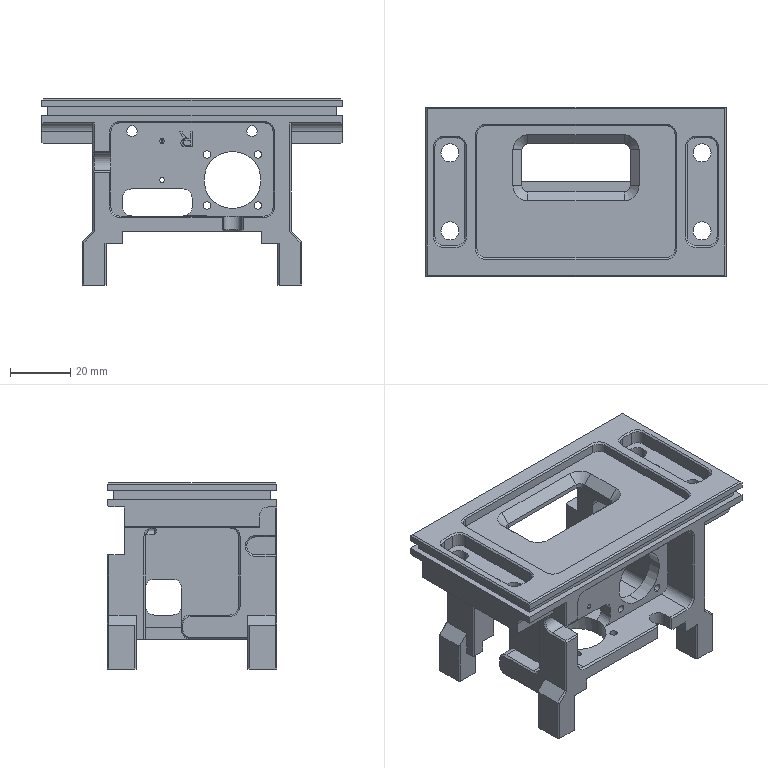NC program | Mastercam | posted with a generic post | part box 100 x 56.5 x 62 mm
Lines 1 to 33 of 47040:
%
O0000()
(MATERIAL - ALUMINUM MM - 2024)
( T20 | 63 FEM | H20 )
( T13 | 16 FEM | H13 | XY STOCK TO LEAVE - .15 | Z STOCK TO LEAVE - 0. )
( T16 | 16 FEM | H16 | XY STOCK TO LEAVE - .02 | Z STOCK TO LEAVE - 0. )
( T6 | 6 FEM | H6 | XY STOCK TO LEAVE - .1 | Z STOCK TO LEAVE - .1 )
( T2 | 2 FEM | H2 | XY STOCK TO LEAVE - .07 | Z STOCK TO LEAVE - .05 )
( T5 | 4 CHM | H5 )
( T11 | 12 FEM | H11 | XY STOCK TO LEAVE - .1 | Z STOCK TO LEAVE - .1 )
( T12 | 12 FEM | H12 )
( T14 | 6 FEM | H14 | XY STOCK TO LEAVE - .1 | Z STOCK TO LEAVE - .1 )
( T15 | 4 FEM | H15 | XY STOCK TO LEAVE - .07 | Z STOCK TO LEAVE - .05 )
( T3 | 3 FEM | H3 | XY STOCK TO LEAVE - .1 | Z STOCK TO LEAVE - 0. )
( T17 | 14 CHM | H17 )
( T4 | 4 FEM | H4 | XY STOCK TO LEAVE - .07 | Z STOCK TO LEAVE - 0. )
( T18 | 6 FEM | H18 | XY STOCK TO LEAVE - -.01 | Z STOCK TO LEAVE - 0. )
N100 G21
N110 G0 G17 G40 G49 G80 G90
N120 T20 M6
N130 G0 G90 G54 X-101.6 Y23.248 A0. S4000 M3
N140 G43 H20 Z20. M8
N150 Z1.
N160 G1 Z0. F600.
N170 X70.1 F1000.
N180 G2 X93.348 Y0. I0. J-23.248
N190 X70.1 Y-23.248 I-23.248 J0.
N200 G1 X-101.6
N210 G0 Z20.
N220 M5
N230 G91 G28 Z0. M9
N240 A0.
N250 M01